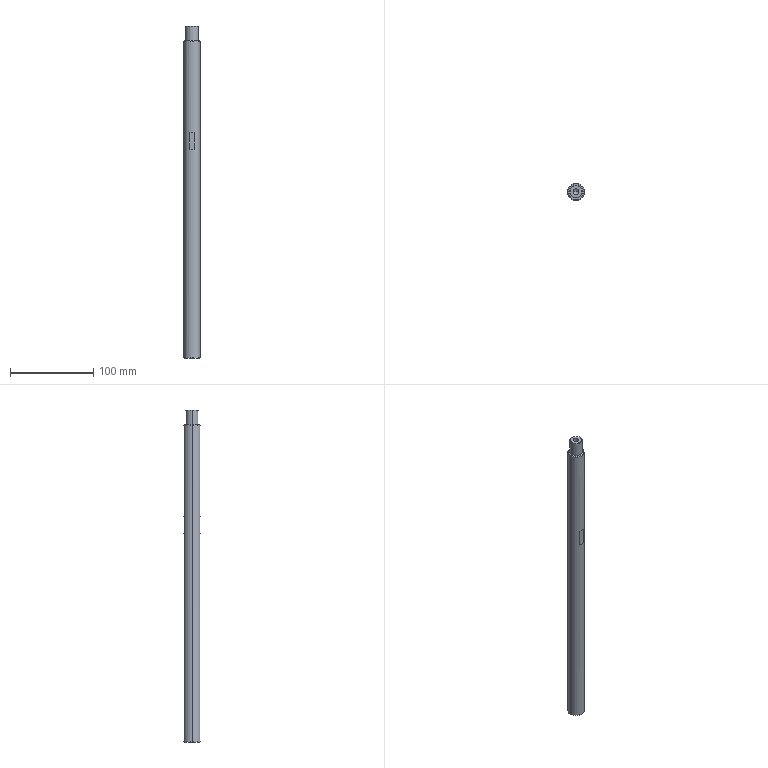Part | STEP file | 11-FG-SJ01611 | 1 solid | 27 faces | box 20 x 20 x 400 mm | volume 121597 mm3 | cone 10 | plane 9 | cylinder 8 | commonest cylinder face diameters 6.8 x4 15 x2 20 x2
STEP:
#1=CARTESIAN_POINT('',(7.,0.,400.));
#2=VERTEX_POINT('',#1);
#3=CARTESIAN_POINT('',(-7.,0.,400.));
#4=VERTEX_POINT('',#3);
#5=CARTESIAN_POINT('',(0.,0.,400.));
#6=DIRECTION('',(0.,0.,1.));
#7=DIRECTION('',(1.,0.,0.));
#8=AXIS2_PLACEMENT_3D('',#5,#6,#7);
#9=CIRCLE('',#8,7.);
#10=EDGE_CURVE('',#2,#4,#9,.T.);
#11=ORIENTED_EDGE('',*,*,#10,.F.);
#12=CARTESIAN_POINT('',(7.5,0.,399.5));
#13=VERTEX_POINT('',#12);
#14=CARTESIAN_POINT('',(7.,0.,400.));
#15=DIRECTION('',(0.7071,0.,-0.7071));
#16=VECTOR('',#15,1000.);
#17=LINE('',#14,#16);
#18=EDGE_CURVE('',#2,#13,#17,.T.);
#19=ORIENTED_EDGE('',*,*,#18,.T.);
#20=CARTESIAN_POINT('',(-7.5,0.,399.5));
#21=VERTEX_POINT('',#20);
#22=CARTESIAN_POINT('',(0.,0.,399.5));
#23=DIRECTION('',(0.,0.,-1.));
#24=DIRECTION('',(1.,0.,0.));
#25=AXIS2_PLACEMENT_3D('',#22,#23,#24);
#26=CIRCLE('',#25,7.5);
#27=EDGE_CURVE('',#21,#13,#26,.T.);
#28=ORIENTED_EDGE('',*,*,#27,.F.);
#29=CARTESIAN_POINT('',(-7.,0.,400.));
#30=DIRECTION('',(-0.7071,0.,-0.7071));
#31=VECTOR('',#30,1000.);
#32=LINE('',#29,#31);
#33=EDGE_CURVE('',#4,#21,#32,.T.);
#34=ORIENTED_EDGE('',*,*,#33,.F.);
#35=EDGE_LOOP('',(#11,#19,#28,#34));
#36=FACE_OUTER_BOUND('',#35,.T.);
#37=CARTESIAN_POINT('',(0.,0.,400.));
#38=DIRECTION('',(0.,0.,-1.));
#39=DIRECTION('',(-1.,0.,0.));
#40=AXIS2_PLACEMENT_3D('',#37,#38,#39);
#41=CONICAL_SURFACE('',#40,7.,0.7854);
#42=ADVANCED_FACE('',(#36),#41,.T.);
#43=CARTESIAN_POINT('',(-9.5,0.,0.));
#44=VERTEX_POINT('',#43);
#45=CARTESIAN_POINT('',(9.5,0.,0.));
#46=VERTEX_POINT('',#45);
#47=CARTESIAN_POINT('',(0.,0.,0.));
#48=DIRECTION('',(0.,0.,-1.));
#49=DIRECTION('',(1.,0.,0.));
#50=AXIS2_PLACEMENT_3D('',#47,#48,#49);
#51=CIRCLE('',#50,9.5);
#52=EDGE_CURVE('',#44,#46,#51,.T.);
#53=ORIENTED_EDGE('',*,*,#52,.F.);
#54=CARTESIAN_POINT('',(-10.,0.,0.5));
#55=VERTEX_POINT('',#54);
#56=CARTESIAN_POINT('',(-10.,0.,0.5));
#57=DIRECTION('',(-0.7071,0.,0.7071));
#58=VECTOR('',#57,1000.);
#59=LINE('',#56,#58);
#60=EDGE_CURVE('',#44,#55,#59,.T.);
#61=ORIENTED_EDGE('',*,*,#60,.T.);
#62=CARTESIAN_POINT('',(10.,0.,0.5));
#63=VERTEX_POINT('',#62);
#64=CARTESIAN_POINT('',(0.,0.,0.5));
#65=DIRECTION('',(0.,0.,1.));
#66=DIRECTION('',(1.,0.,0.));
#67=AXIS2_PLACEMENT_3D('',#64,#65,#66);
#68=CIRCLE('',#67,10.);
#69=EDGE_CURVE('',#63,#55,#68,.T.);
#70=ORIENTED_EDGE('',*,*,#69,.F.);
#71=CARTESIAN_POINT('',(10.,0.,0.5));
#72=DIRECTION('',(0.7071,0.,0.7071));
#73=VECTOR('',#72,1000.);
#74=LINE('',#71,#73);
#75=EDGE_CURVE('',#46,#63,#74,.T.);
#76=ORIENTED_EDGE('',*,*,#75,.F.);
#77=EDGE_LOOP('',(#53,#61,#70,#76));
#78=FACE_OUTER_BOUND('',#77,.T.);
#79=CARTESIAN_POINT('',(0.,0.,0.5));
#80=DIRECTION('',(0.,0.,1.));
#81=DIRECTION('',(1.,0.,0.));
#82=AXIS2_PLACEMENT_3D('',#79,#80,#81);
#83=CONICAL_SURFACE('',#82,10.,0.7854);
#84=ADVANCED_FACE('',(#78),#83,.T.);
#85=CARTESIAN_POINT('',(9.5,0.,382.));
#86=VERTEX_POINT('',#85);
#87=CARTESIAN_POINT('',(-9.5,0.,382.));
#88=VERTEX_POINT('',#87);
#89=CARTESIAN_POINT('',(0.,0.,382.));
#90=DIRECTION('',(0.,0.,1.));
#91=DIRECTION('',(1.,0.,0.));
#92=AXIS2_PLACEMENT_3D('',#89,#90,#91);
#93=CIRCLE('',#92,9.5);
#94=EDGE_CURVE('',#86,#88,#93,.T.);
#95=ORIENTED_EDGE('',*,*,#94,.F.);
#96=CARTESIAN_POINT('',(10.,0.,381.5));
#97=VERTEX_POINT('',#96);
#98=CARTESIAN_POINT('',(9.5,0.,382.));
#99=DIRECTION('',(0.7071,0.,-0.7071));
#100=VECTOR('',#99,1000.);
#101=LINE('',#98,#100);
#102=EDGE_CURVE('',#86,#97,#101,.T.);
#103=ORIENTED_EDGE('',*,*,#102,.T.);
#104=CARTESIAN_POINT('',(-10.,0.,381.5));
#105=VERTEX_POINT('',#104);
#106=CARTESIAN_POINT('',(0.,0.,381.5));
#107=DIRECTION('',(0.,0.,-1.));
#108=DIRECTION('',(1.,0.,0.));
#109=AXIS2_PLACEMENT_3D('',#106,#107,#108);
#110=CIRCLE('',#109,10.);
#111=EDGE_CURVE('',#105,#97,#110,.T.);
#112=ORIENTED_EDGE('',*,*,#111,.F.);
#113=CARTESIAN_POINT('',(-9.5,0.,382.));
#114=DIRECTION('',(-0.7071,0.,-0.7071));
#115=VECTOR('',#114,1000.);
#116=LINE('',#113,#115);
#117=EDGE_CURVE('',#88,#105,#116,.T.);
#118=ORIENTED_EDGE('',*,*,#117,.F.);
#119=EDGE_LOOP('',(#95,#103,#112,#118));
#120=FACE_OUTER_BOUND('',#119,.T.);
#121=CARTESIAN_POINT('',(0.,0.,382.));
#122=DIRECTION('',(0.,0.,-1.));
#123=DIRECTION('',(-1.,0.,0.));
#124=AXIS2_PLACEMENT_3D('',#121,#122,#123);
#125=CONICAL_SURFACE('',#124,9.5,0.7854);
#126=ADVANCED_FACE('',(#120),#125,.T.);
#127=CARTESIAN_POINT('',(-3.4,0.,380.2));
#128=VERTEX_POINT('',#127);
#129=CARTESIAN_POINT('',(3.4,0.,380.2));
#130=VERTEX_POINT('',#129);
#131=CARTESIAN_POINT('',(0.,0.,380.2));
#132=DIRECTION('',(0.,0.,1.));
#133=DIRECTION('',(1.,0.,0.));
#134=AXIS2_PLACEMENT_3D('',#131,#132,#133);
#135=CIRCLE('',#134,3.4);
#136=EDGE_CURVE('',#128,#130,#135,.T.);
#137=ORIENTED_EDGE('',*,*,#136,.F.);
#138=CARTESIAN_POINT('',(-3.4,0.,400.));
#139=VERTEX_POINT('',#138);
#140=CARTESIAN_POINT('',(-3.4,0.,400.));
#141=DIRECTION('',(0.,0.,1.));
#142=VECTOR('',#141,1000.);
#143=LINE('',#140,#142);
#144=EDGE_CURVE('',#128,#139,#143,.T.);
#145=ORIENTED_EDGE('',*,*,#144,.T.);
#146=CARTESIAN_POINT('',(3.4,0.,400.));
#147=VERTEX_POINT('',#146);
#148=CARTESIAN_POINT('',(0.,0.,400.));
#149=DIRECTION('',(0.,0.,1.));
#150=DIRECTION('',(1.,0.,0.));
#151=AXIS2_PLACEMENT_3D('',#148,#149,#150);
#152=CIRCLE('',#151,3.4);
#153=EDGE_CURVE('',#139,#147,#152,.T.);
#154=ORIENTED_EDGE('',*,*,#153,.T.);
#155=CARTESIAN_POINT('',(3.4,0.,400.));
#156=DIRECTION('',(0.,0.,1.));
#157=VECTOR('',#156,1000.);
#158=LINE('',#155,#157);
#159=EDGE_CURVE('',#130,#147,#158,.T.);
#160=ORIENTED_EDGE('',*,*,#159,.F.);
#161=EDGE_LOOP('',(#137,#145,#154,#160));
#162=FACE_OUTER_BOUND('',#161,.T.);
#163=CARTESIAN_POINT('',(0.,0.,400.));
#164=DIRECTION('',(0.,0.,1.));
#165=DIRECTION('',(1.,0.,0.));
#166=AXIS2_PLACEMENT_3D('',#163,#164,#165);
#167=CYLINDRICAL_SURFACE('',#166,3.4);
#168=ADVANCED_FACE('',(#162),#167,.F.);
#169=CARTESIAN_POINT('',(0.,0.,378.157));
#170=VERTEX_POINT('',#169);
#171=CARTESIAN_POINT('',(3.4,0.,380.2));
#172=DIRECTION('',(0.8572,0.,0.515));
#173=VECTOR('',#172,1000.);
#174=LINE('',#171,#173);
#175=EDGE_CURVE('',#170,#130,#174,.T.);
#176=ORIENTED_EDGE('',*,*,#175,.F.);
#177=CARTESIAN_POINT('',(-3.4,0.,380.2));
#178=DIRECTION('',(-0.8572,0.,0.515));
#179=VECTOR('',#178,1000.);
#180=LINE('',#177,#179);
#181=EDGE_CURVE('',#170,#128,#180,.T.);
#182=ORIENTED_EDGE('',*,*,#181,.T.);
#183=ORIENTED_EDGE('',*,*,#136,.T.);
#184=EDGE_LOOP('',(#176,#182,#183));
#185=FACE_OUTER_BOUND('',#184,.T.);
#186=CARTESIAN_POINT('',(0.,0.,380.2));
#187=DIRECTION('',(0.,0.,1.));
#188=DIRECTION('',(1.,0.,0.));
#189=AXIS2_PLACEMENT_3D('',#186,#187,#188);
#190=CONICAL_SURFACE('',#189,3.4,1.03);
#191=ADVANCED_FACE('',(#185),#190,.F.);
#192=CARTESIAN_POINT('',(7.5,0.,382.));
#193=VERTEX_POINT('',#192);
#194=CARTESIAN_POINT('',(-7.5,0.,382.));
#195=VERTEX_POINT('',#194);
#196=CARTESIAN_POINT('',(0.,0.,382.));
#197=DIRECTION('',(0.,0.,1.));
#198=DIRECTION('',(1.,0.,0.));
#199=AXIS2_PLACEMENT_3D('',#196,#197,#198);
#200=CIRCLE('',#199,7.5);
#201=EDGE_CURVE('',#193,#195,#200,.T.);
#202=ORIENTED_EDGE('',*,*,#201,.T.);
#203=CARTESIAN_POINT('',(-7.5,0.,382.));
#204=DIRECTION('',(0.,0.,1.));
#205=VECTOR('',#204,1000.);
#206=LINE('',#203,#205);
#207=EDGE_CURVE('',#195,#21,#206,.T.);
#208=ORIENTED_EDGE('',*,*,#207,.T.);
#209=ORIENTED_EDGE('',*,*,#27,.T.);
#210=CARTESIAN_POINT('',(7.5,0.,382.));
#211=DIRECTION('',(0.,0.,1.));
#212=VECTOR('',#211,1000.);
#213=LINE('',#210,#212);
#214=EDGE_CURVE('',#193,#13,#213,.T.);
#215=ORIENTED_EDGE('',*,*,#214,.F.);
#216=EDGE_LOOP('',(#202,#208,#209,#215));
#217=FACE_OUTER_BOUND('',#216,.T.);
#218=CARTESIAN_POINT('',(0.,0.,382.));
#219=DIRECTION('',(0.,0.,1.));
#220=DIRECTION('',(1.,0.,0.));
#221=AXIS2_PLACEMENT_3D('',#218,#219,#220);
#222=CYLINDRICAL_SURFACE('',#221,7.5);
#223=ADVANCED_FACE('',(#217),#222,.T.);
#224=CARTESIAN_POINT('',(3.4,0.,19.8));
#225=VERTEX_POINT('',#224);
#226=CARTESIAN_POINT('',(-3.4,0.,19.8));
#227=VERTEX_POINT('',#226);
#228=CARTESIAN_POINT('',(0.,0.,19.8));
#229=DIRECTION('',(0.,0.,-1.));
#230=DIRECTION('',(-1.,0.,0.));
#231=AXIS2_PLACEMENT_3D('',#228,#229,#230);
#232=CIRCLE('',#231,3.4);
#233=EDGE_CURVE('',#225,#227,#232,.T.);
#234=ORIENTED_EDGE('',*,*,#233,.F.);
#235=CARTESIAN_POINT('',(3.4,0.,0.));
#236=VERTEX_POINT('',#235);
#237=CARTESIAN_POINT('',(3.4,0.,0.));
#238=DIRECTION('',(0.,0.,-1.));
#239=VECTOR('',#238,1000.);
#240=LINE('',#237,#239);
#241=EDGE_CURVE('',#225,#236,#240,.T.);
#242=ORIENTED_EDGE('',*,*,#241,.T.);
#243=CARTESIAN_POINT('',(-3.4,0.,0.));
#244=VERTEX_POINT('',#243);
#245=CARTESIAN_POINT('',(0.,0.,0.));
#246=DIRECTION('',(0.,0.,-1.));
#247=DIRECTION('',(-1.,0.,0.));
#248=AXIS2_PLACEMENT_3D('',#245,#246,#247);
#249=CIRCLE('',#248,3.4);
#250=EDGE_CURVE('',#236,#244,#249,.T.);
#251=ORIENTED_EDGE('',*,*,#250,.T.);
#252=CARTESIAN_POINT('',(-3.4,0.,0.));
#253=DIRECTION('',(0.,0.,-1.));
#254=VECTOR('',#253,1000.);
#255=LINE('',#252,#254);
#256=EDGE_CURVE('',#227,#244,#255,.T.);
#257=ORIENTED_EDGE('',*,*,#256,.F.);
#258=EDGE_LOOP('',(#234,#242,#251,#257));
#259=FACE_OUTER_BOUND('',#258,.T.);
#260=CARTESIAN_POINT('',(0.,0.,0.));
#261=DIRECTION('',(0.,0.,-1.));
#262=DIRECTION('',(-1.,0.,0.));
#263=AXIS2_PLACEMENT_3D('',#260,#261,#262);
#264=CYLINDRICAL_SURFACE('',#263,3.4);
#265=ADVANCED_FACE('',(#259),#264,.F.);
#266=CARTESIAN_POINT('',(0.,0.,21.843));
#267=VERTEX_POINT('',#266);
#268=CARTESIAN_POINT('',(-3.4,0.,19.8));
#269=DIRECTION('',(-0.8572,0.,-0.515));
#270=VECTOR('',#269,1000.);
#271=LINE('',#268,#270);
#272=EDGE_CURVE('',#267,#227,#271,.T.);
#273=ORIENTED_EDGE('',*,*,#272,.F.);
#274=CARTESIAN_POINT('',(3.4,0.,19.8));
#275=DIRECTION('',(0.8572,0.,-0.515));
#276=VECTOR('',#275,1000.);
#277=LINE('',#274,#276);
#278=EDGE_CURVE('',#267,#225,#277,.T.);
#279=ORIENTED_EDGE('',*,*,#278,.T.);
#280=ORIENTED_EDGE('',*,*,#233,.T.);
#281=EDGE_LOOP('',(#273,#279,#280));
#282=FACE_OUTER_BOUND('',#281,.T.);
#283=CARTESIAN_POINT('',(0.,0.,19.8));
#284=DIRECTION('',(0.,0.,-1.));
#285=DIRECTION('',(-1.,0.,0.));
#286=AXIS2_PLACEMENT_3D('',#283,#284,#285);
#287=CONICAL_SURFACE('',#286,3.4,1.03);
#288=ADVANCED_FACE('',(#282),#287,.F.);
#289=CARTESIAN_POINT('',(3.122,9.5,251.5));
#290=VERTEX_POINT('',#289);
#291=CARTESIAN_POINT('',(-3.122,9.5,251.5));
#292=VERTEX_POINT('',#291);
#293=CARTESIAN_POINT('',(0.,0.,251.5));
#294=DIRECTION('',(0.,0.,1.));
#295=DIRECTION('',(1.,0.,0.));
#296=AXIS2_PLACEMENT_3D('',#293,#294,#295);
#297=CIRCLE('',#296,10.);
#298=EDGE_CURVE('',#290,#292,#297,.T.);
#299=ORIENTED_EDGE('',*,*,#298,.F.);
#300=CARTESIAN_POINT('',(3.122,9.5,271.5));
#301=VERTEX_POINT('',#300);
#302=CARTESIAN_POINT('',(3.122,9.5,251.5));
#303=DIRECTION('',(0.,0.,1.));
#304=VECTOR('',#303,1000.);
#305=LINE('',#302,#304);
#306=EDGE_CURVE('',#290,#301,#305,.T.);
#307=ORIENTED_EDGE('',*,*,#306,.T.);
#308=CARTESIAN_POINT('',(-3.122,9.5,271.5));
#309=VERTEX_POINT('',#308);
#310=CARTESIAN_POINT('',(0.,0.,271.5));
#311=DIRECTION('',(0.,0.,1.));
#312=DIRECTION('',(1.,0.,0.));
#313=AXIS2_PLACEMENT_3D('',#310,#311,#312);
#314=CIRCLE('',#313,10.);
#315=EDGE_CURVE('',#301,#309,#314,.T.);
#316=ORIENTED_EDGE('',*,*,#315,.T.);
#317=CARTESIAN_POINT('',(-3.122,9.5,251.5));
#318=DIRECTION('',(0.,0.,1.));
#319=VECTOR('',#318,1000.);
#320=LINE('',#317,#319);
#321=EDGE_CURVE('',#292,#309,#320,.T.);
#322=ORIENTED_EDGE('',*,*,#321,.F.);
#323=EDGE_LOOP('',(#299,#307,#316,#322));
#324=FACE_BOUND('',#323,.T.);
#325=ORIENTED_EDGE('',*,*,#111,.T.);
#326=CARTESIAN_POINT('',(10.,0.,400.));
#327=DIRECTION('',(0.,0.,-1.));
#328=VECTOR('',#327,1000.);
#329=LINE('',#326,#328);
#330=EDGE_CURVE('',#97,#63,#329,.T.);
#331=ORIENTED_EDGE('',*,*,#330,.T.);
#332=ORIENTED_EDGE('',*,*,#69,.T.);
#333=CARTESIAN_POINT('',(-10.,0.,400.));
#334=DIRECTION('',(0.,0.,-1.));
#335=VECTOR('',#334,1000.);
#336=LINE('',#333,#335);
#337=EDGE_CURVE('',#105,#55,#336,.T.);
#338=ORIENTED_EDGE('',*,*,#337,.F.);
#339=EDGE_LOOP('',(#325,#331,#332,#338));
#340=FACE_OUTER_BOUND('',#339,.T.);
#341=CARTESIAN_POINT('',(0.,0.,400.));
#342=DIRECTION('',(0.,0.,-1.));
#343=DIRECTION('',(-1.,0.,0.));
#344=AXIS2_PLACEMENT_3D('',#341,#342,#343);
#345=CYLINDRICAL_SURFACE('',#344,10.);
#346=ADVANCED_FACE('',(#324,#340),#345,.T.);
#347=ORIENTED_EDGE('',*,*,#330,.F.);
#348=CARTESIAN_POINT('',(0.,0.,381.5));
#349=DIRECTION('',(0.,0.,-1.));
#350=DIRECTION('',(1.,0.,0.));
#351=AXIS2_PLACEMENT_3D('',#348,#349,#350);
#352=CIRCLE('',#351,10.);
#353=EDGE_CURVE('',#97,#105,#352,.T.);
#354=ORIENTED_EDGE('',*,*,#353,.T.);
#355=ORIENTED_EDGE('',*,*,#337,.T.);
#356=CARTESIAN_POINT('',(0.,0.,0.5));
#357=DIRECTION('',(0.,0.,1.));
#358=DIRECTION('',(1.,0.,0.));
#359=AXIS2_PLACEMENT_3D('',#356,#357,#358);
#360=CIRCLE('',#359,10.);
#361=EDGE_CURVE('',#55,#63,#360,.T.);
#362=ORIENTED_EDGE('',*,*,#361,.T.);
#363=EDGE_LOOP('',(#347,#354,#355,#362));
#364=FACE_OUTER_BOUND('',#363,.T.);
#365=CARTESIAN_POINT('',(-3.122,-9.5,251.5));
#366=VERTEX_POINT('',#365);
#367=CARTESIAN_POINT('',(3.122,-9.5,251.5));
#368=VERTEX_POINT('',#367);
#369=CARTESIAN_POINT('',(0.,0.,251.5));
#370=DIRECTION('',(0.,0.,1.));
#371=DIRECTION('',(1.,0.,0.));
#372=AXIS2_PLACEMENT_3D('',#369,#370,#371);
#373=CIRCLE('',#372,10.);
#374=EDGE_CURVE('',#366,#368,#373,.T.);
#375=ORIENTED_EDGE('',*,*,#374,.F.);
#376=CARTESIAN_POINT('',(-3.122,-9.5,271.5));
#377=VERTEX_POINT('',#376);
#378=CARTESIAN_POINT('',(-3.122,-9.5,251.5));
#379=DIRECTION('',(0.,0.,1.));
#380=VECTOR('',#379,1000.);
#381=LINE('',#378,#380);
#382=EDGE_CURVE('',#366,#377,#381,.T.);
#383=ORIENTED_EDGE('',*,*,#382,.T.);
#384=CARTESIAN_POINT('',(3.122,-9.5,271.5));
#385=VERTEX_POINT('',#384);
#386=CARTESIAN_POINT('',(0.,0.,271.5));
#387=DIRECTION('',(0.,0.,1.));
#388=DIRECTION('',(1.,0.,0.));
#389=AXIS2_PLACEMENT_3D('',#386,#387,#388);
#390=CIRCLE('',#389,10.);
#391=EDGE_CURVE('',#377,#385,#390,.T.);
#392=ORIENTED_EDGE('',*,*,#391,.T.);
#393=CARTESIAN_POINT('',(3.122,-9.5,251.5));
#394=DIRECTION('',(0.,0.,1.));
#395=VECTOR('',#394,1000.);
#396=LINE('',#393,#395);
#397=EDGE_CURVE('',#368,#385,#396,.T.);
#398=ORIENTED_EDGE('',*,*,#397,.F.);
#399=EDGE_LOOP('',(#375,#383,#392,#398));
#400=FACE_BOUND('',#399,.T.);
#401=CARTESIAN_POINT('',(0.,0.,400.));
#402=DIRECTION('',(0.,0.,-1.));
#403=DIRECTION('',(-1.,0.,0.));
#404=AXIS2_PLACEMENT_3D('',#401,#402,#403);
#405=CYLINDRICAL_SURFACE('',#404,10.);
#406=ADVANCED_FACE('',(#364,#400),#405,.T.);
#407=CARTESIAN_POINT('',(0.,0.,0.));
#408=DIRECTION('',(0.,0.,-1.));
#409=DIRECTION('',(1.,0.,0.));
#410=AXIS2_PLACEMENT_3D('',#407,#408,#409);
#411=CIRCLE('',#410,9.5);
#412=EDGE_CURVE('',#46,#44,#411,.T.);
#413=ORIENTED_EDGE('',*,*,#412,.T.);
#414=ORIENTED_EDGE('',*,*,#52,.T.);
#415=EDGE_LOOP('',(#413,#414));
#416=FACE_OUTER_BOUND('',#415,.T.);
#417=CARTESIAN_POINT('',(0.,0.,0.));
#418=DIRECTION('',(0.,0.,-1.));
#419=DIRECTION('',(-1.,0.,0.));
#420=AXIS2_PLACEMENT_3D('',#417,#418,#419);
#421=CIRCLE('',#420,3.4);
#422=EDGE_CURVE('',#244,#236,#421,.T.);
#423=ORIENTED_EDGE('',*,*,#422,.F.);
#424=ORIENTED_EDGE('',*,*,#250,.F.);
#425=EDGE_LOOP('',(#423,#424));
#426=FACE_BOUND('',#425,.T.);
#427=CARTESIAN_POINT('',(0.,0.,0.));
#428=DIRECTION('',(0.,0.,1.));
#429=DIRECTION('',(1.,0.,0.));
#430=AXIS2_PLACEMENT_3D('',#427,#428,#429);
#431=PLANE('',#430);
#432=ADVANCED_FACE('',(#416,#426),#431,.F.);
#433=CARTESIAN_POINT('',(-3.122,9.5,271.5));
#434=DIRECTION('',(1.,0.,0.));
#435=VECTOR('',#434,1000.);
#436=LINE('',#433,#435);
#437=EDGE_CURVE('',#309,#301,#436,.T.);
#438=ORIENTED_EDGE('',*,*,#437,.T.);
#439=ORIENTED_EDGE('',*,*,#306,.F.);
#440=CARTESIAN_POINT('',(-3.122,9.5,251.5));
#441=DIRECTION('',(1.,0.,0.));
#442=VECTOR('',#441,1000.);
#443=LINE('',#440,#442);
#444=EDGE_CURVE('',#292,#290,#443,.T.);
#445=ORIENTED_EDGE('',*,*,#444,.F.);
#446=ORIENTED_EDGE('',*,*,#321,.T.);
#447=EDGE_LOOP('',(#438,#439,#445,#446));
#448=FACE_OUTER_BOUND('',#447,.T.);
#449=CARTESIAN_POINT('',(-3.122,9.5,251.5));
#450=DIRECTION('',(0.,-1.,0.));
#451=DIRECTION('',(0.,0.,-1.));
#452=AXIS2_PLACEMENT_3D('',#449,#450,#451);
#453=PLANE('',#452);
#454=ADVANCED_FACE('',(#448),#453,.F.);
#455=ORIENTED_EDGE('',*,*,#298,.T.);
#456=ORIENTED_EDGE('',*,*,#444,.T.);
#457=EDGE_LOOP('',(#455,#456));
#458=FACE_OUTER_BOUND('',#457,.T.);
#459=CARTESIAN_POINT('',(0.,0.,251.5));
#460=DIRECTION('',(0.,0.,1.));
#461=DIRECTION('',(1.,0.,0.));
#462=AXIS2_PLACEMENT_3D('',#459,#460,#461);
#463=PLANE('',#462);
#464=ADVANCED_FACE('',(#458),#463,.T.);
#465=ORIENTED_EDGE('',*,*,#315,.F.);
#466=ORIENTED_EDGE('',*,*,#437,.F.);
#467=EDGE_LOOP('',(#465,#466));
#468=FACE_OUTER_BOUND('',#467,.T.);
#469=CARTESIAN_POINT('',(0.,0.,271.5));
#470=DIRECTION('',(0.,0.,1.));
#471=DIRECTION('',(1.,0.,0.));
#472=AXIS2_PLACEMENT_3D('',#469,#470,#471);
#473=PLANE('',#472);
#474=ADVANCED_FACE('',(#468),#473,.F.);
#475=CARTESIAN_POINT('',(-3.122,-9.5,271.5));
#476=DIRECTION('',(-1.,0.,0.));
#477=VECTOR('',#476,1000.);
#478=LINE('',#475,#477);
#479=EDGE_CURVE('',#385,#377,#478,.T.);
#480=ORIENTED_EDGE('',*,*,#479,.T.);
#481=ORIENTED_EDGE('',*,*,#382,.F.);
#482=CARTESIAN_POINT('',(-3.122,-9.5,251.5));
#483=DIRECTION('',(-1.,0.,0.));
#484=VECTOR('',#483,1000.);
#485=LINE('',#482,#484);
#486=EDGE_CURVE('',#368,#366,#485,.T.);
#487=ORIENTED_EDGE('',*,*,#486,.F.);
#488=ORIENTED_EDGE('',*,*,#397,.T.);
#489=EDGE_LOOP('',(#480,#481,#487,#488));
#490=FACE_OUTER_BOUND('',#489,.T.);
#491=CARTESIAN_POINT('',(-3.122,-9.5,251.5));
#492=DIRECTION('',(0.,1.,0.));
#493=DIRECTION('',(0.,0.,1.));
#494=AXIS2_PLACEMENT_3D('',#491,#492,#493);
#495=PLANE('',#494);
#496=ADVANCED_FACE('',(#490),#495,.F.);
#497=ORIENTED_EDGE('',*,*,#374,.T.);
#498=ORIENTED_EDGE('',*,*,#486,.T.);
#499=EDGE_LOOP('',(#497,#498));
#500=FACE_OUTER_BOUND('',#499,.T.);
#501=CARTESIAN_POINT('',(0.,0.,251.5));
#502=DIRECTION('',(0.,0.,1.));
#503=DIRECTION('',(1.,0.,0.));
#504=AXIS2_PLACEMENT_3D('',#501,#502,#503);
#505=PLANE('',#504);
#506=ADVANCED_FACE('',(#500),#505,.T.);
#507=ORIENTED_EDGE('',*,*,#391,.F.);
#508=ORIENTED_EDGE('',*,*,#479,.F.);
#509=EDGE_LOOP('',(#507,#508));
#510=FACE_OUTER_BOUND('',#509,.T.);
#511=CARTESIAN_POINT('',(0.,0.,271.5));
#512=DIRECTION('',(0.,0.,1.));
#513=DIRECTION('',(1.,0.,0.));
#514=AXIS2_PLACEMENT_3D('',#511,#512,#513);
#515=PLANE('',#514);
#516=ADVANCED_FACE('',(#510),#515,.F.);
#517=ORIENTED_EDGE('',*,*,#278,.F.);
#518=ORIENTED_EDGE('',*,*,#272,.T.);
#519=CARTESIAN_POINT('',(0.,0.,19.8));
#520=DIRECTION('',(0.,0.,-1.));
#521=DIRECTION('',(-1.,0.,0.));
#522=AXIS2_PLACEMENT_3D('',#519,#520,#521);
#523=CIRCLE('',#522,3.4);
#524=EDGE_CURVE('',#227,#225,#523,.T.);
#525=ORIENTED_EDGE('',*,*,#524,.T.);
#526=EDGE_LOOP('',(#517,#518,#525));
#527=FACE_OUTER_BOUND('',#526,.T.);
#528=CARTESIAN_POINT('',(0.,0.,19.8));
#529=DIRECTION('',(0.,0.,-1.));
#530=DIRECTION('',(-1.,0.,0.));
#531=AXIS2_PLACEMENT_3D('',#528,#529,#530);
#532=CONICAL_SURFACE('',#531,3.4,1.03);
#533=ADVANCED_FACE('',(#527),#532,.F.);
#534=ORIENTED_EDGE('',*,*,#241,.F.);
#535=ORIENTED_EDGE('',*,*,#524,.F.);
#536=ORIENTED_EDGE('',*,*,#256,.T.);
#537=ORIENTED_EDGE('',*,*,#422,.T.);
#538=EDGE_LOOP('',(#534,#535,#536,#537));
#539=FACE_OUTER_BOUND('',#538,.T.);
#540=CARTESIAN_POINT('',(0.,0.,0.));
#541=DIRECTION('',(0.,0.,-1.));
#542=DIRECTION('',(-1.,0.,0.));
#543=AXIS2_PLACEMENT_3D('',#540,#541,#542);
#544=CYLINDRICAL_SURFACE('',#543,3.4);
#545=ADVANCED_FACE('',(#539),#544,.F.);
#546=CARTESIAN_POINT('',(0.,0.,382.));
#547=DIRECTION('',(0.,0.,1.));
#548=DIRECTION('',(1.,0.,0.));
#549=AXIS2_PLACEMENT_3D('',#546,#547,#548);
#550=CIRCLE('',#549,9.5);
#551=EDGE_CURVE('',#88,#86,#550,.T.);
#552=ORIENTED_EDGE('',*,*,#551,.T.);
#553=ORIENTED_EDGE('',*,*,#94,.T.);
#554=EDGE_LOOP('',(#552,#553));
#555=FACE_OUTER_BOUND('',#554,.T.);
#556=ORIENTED_EDGE('',*,*,#201,.F.);
#557=CARTESIAN_POINT('',(0.,0.,382.));
#558=DIRECTION('',(0.,0.,1.));
#559=DIRECTION('',(1.,0.,0.));
#560=AXIS2_PLACEMENT_3D('',#557,#558,#559);
#561=CIRCLE('',#560,7.5);
#562=EDGE_CURVE('',#195,#193,#561,.T.);
#563=ORIENTED_EDGE('',*,*,#562,.F.);
#564=EDGE_LOOP('',(#556,#563));
#565=FACE_BOUND('',#564,.T.);
#566=CARTESIAN_POINT('',(0.,0.,382.));
#567=DIRECTION('',(0.,0.,1.));
#568=DIRECTION('',(1.,0.,0.));
#569=AXIS2_PLACEMENT_3D('',#566,#567,#568);
#570=PLANE('',#569);
#571=ADVANCED_FACE('',(#555,#565),#570,.T.);
#572=ORIENTED_EDGE('',*,*,#207,.F.);
#573=ORIENTED_EDGE('',*,*,#562,.T.);
#574=ORIENTED_EDGE('',*,*,#214,.T.);
#575=CARTESIAN_POINT('',(0.,0.,399.5));
#576=DIRECTION('',(0.,0.,-1.));
#577=DIRECTION('',(1.,0.,0.));
#578=AXIS2_PLACEMENT_3D('',#575,#576,#577);
#579=CIRCLE('',#578,7.5);
#580=EDGE_CURVE('',#13,#21,#579,.T.);
#581=ORIENTED_EDGE('',*,*,#580,.T.);
#582=EDGE_LOOP('',(#572,#573,#574,#581));
#583=FACE_OUTER_BOUND('',#582,.T.);
#584=CARTESIAN_POINT('',(0.,0.,382.));
#585=DIRECTION('',(0.,0.,1.));
#586=DIRECTION('',(1.,0.,0.));
#587=AXIS2_PLACEMENT_3D('',#584,#585,#586);
#588=CYLINDRICAL_SURFACE('',#587,7.5);
#589=ADVANCED_FACE('',(#583),#588,.T.);
#590=ORIENTED_EDGE('',*,*,#181,.F.);
#591=ORIENTED_EDGE('',*,*,#175,.T.);
#592=CARTESIAN_POINT('',(0.,0.,380.2));
#593=DIRECTION('',(0.,0.,1.));
#594=DIRECTION('',(1.,0.,0.));
#595=AXIS2_PLACEMENT_3D('',#592,#593,#594);
#596=CIRCLE('',#595,3.4);
#597=EDGE_CURVE('',#130,#128,#596,.T.);
#598=ORIENTED_EDGE('',*,*,#597,.T.);
#599=EDGE_LOOP('',(#590,#591,#598));
#600=FACE_OUTER_BOUND('',#599,.T.);
#601=CARTESIAN_POINT('',(0.,0.,380.2));
#602=DIRECTION('',(0.,0.,1.));
#603=DIRECTION('',(1.,0.,0.));
#604=AXIS2_PLACEMENT_3D('',#601,#602,#603);
#605=CONICAL_SURFACE('',#604,3.4,1.03);
#606=ADVANCED_FACE('',(#600),#605,.F.);
#607=ORIENTED_EDGE('',*,*,#144,.F.);
#608=ORIENTED_EDGE('',*,*,#597,.F.);
#609=ORIENTED_EDGE('',*,*,#159,.T.);
#610=CARTESIAN_POINT('',(0.,0.,400.));
#611=DIRECTION('',(0.,0.,1.));
#612=DIRECTION('',(1.,0.,0.));
#613=AXIS2_PLACEMENT_3D('',#610,#611,#612);
#614=CIRCLE('',#613,3.4);
#615=EDGE_CURVE('',#147,#139,#614,.T.);
#616=ORIENTED_EDGE('',*,*,#615,.T.);
#617=EDGE_LOOP('',(#607,#608,#609,#616));
#618=FACE_OUTER_BOUND('',#617,.T.);
#619=CARTESIAN_POINT('',(0.,0.,400.));
#620=DIRECTION('',(0.,0.,1.));
#621=DIRECTION('',(1.,0.,0.));
#622=AXIS2_PLACEMENT_3D('',#619,#620,#621);
#623=CYLINDRICAL_SURFACE('',#622,3.4);
#624=ADVANCED_FACE('',(#618),#623,.F.);
#625=CARTESIAN_POINT('',(0.,0.,400.));
#626=DIRECTION('',(0.,0.,1.));
#627=DIRECTION('',(1.,0.,0.));
#628=AXIS2_PLACEMENT_3D('',#625,#626,#627);
#629=CIRCLE('',#628,7.);
#630=EDGE_CURVE('',#4,#2,#629,.T.);
#631=ORIENTED_EDGE('',*,*,#630,.T.);
#632=ORIENTED_EDGE('',*,*,#10,.T.);
#633=EDGE_LOOP('',(#631,#632));
#634=FACE_OUTER_BOUND('',#633,.T.);
#635=ORIENTED_EDGE('',*,*,#615,.F.);
#636=ORIENTED_EDGE('',*,*,#153,.F.);
#637=EDGE_LOOP('',(#635,#636));
#638=FACE_BOUND('',#637,.T.);
#639=CARTESIAN_POINT('',(0.,0.,400.));
#640=DIRECTION('',(0.,0.,1.));
#641=DIRECTION('',(1.,0.,0.));
#642=AXIS2_PLACEMENT_3D('',#639,#640,#641);
#643=PLANE('',#642);
#644=ADVANCED_FACE('',(#634,#638),#643,.T.);
#645=ORIENTED_EDGE('',*,*,#102,.F.);
#646=ORIENTED_EDGE('',*,*,#551,.F.);
#647=ORIENTED_EDGE('',*,*,#117,.T.);
#648=ORIENTED_EDGE('',*,*,#353,.F.);
#649=EDGE_LOOP('',(#645,#646,#647,#648));
#650=FACE_OUTER_BOUND('',#649,.T.);
#651=CARTESIAN_POINT('',(0.,0.,382.));
#652=DIRECTION('',(0.,0.,-1.));
#653=DIRECTION('',(-1.,0.,0.));
#654=AXIS2_PLACEMENT_3D('',#651,#652,#653);
#655=CONICAL_SURFACE('',#654,9.5,0.7854);
#656=ADVANCED_FACE('',(#650),#655,.T.);
#657=ORIENTED_EDGE('',*,*,#60,.F.);
#658=ORIENTED_EDGE('',*,*,#412,.F.);
#659=ORIENTED_EDGE('',*,*,#75,.T.);
#660=ORIENTED_EDGE('',*,*,#361,.F.);
#661=EDGE_LOOP('',(#657,#658,#659,#660));
#662=FACE_OUTER_BOUND('',#661,.T.);
#663=CARTESIAN_POINT('',(0.,0.,0.5));
#664=DIRECTION('',(0.,0.,1.));
#665=DIRECTION('',(1.,0.,0.));
#666=AXIS2_PLACEMENT_3D('',#663,#664,#665);
#667=CONICAL_SURFACE('',#666,10.,0.7854);
#668=ADVANCED_FACE('',(#662),#667,.T.);
#669=ORIENTED_EDGE('',*,*,#18,.F.);
#670=ORIENTED_EDGE('',*,*,#630,.F.);
#671=ORIENTED_EDGE('',*,*,#33,.T.);
#672=ORIENTED_EDGE('',*,*,#580,.F.);
#673=EDGE_LOOP('',(#669,#670,#671,#672));
#674=FACE_OUTER_BOUND('',#673,.T.);
#675=CARTESIAN_POINT('',(0.,0.,400.));
#676=DIRECTION('',(0.,0.,-1.));
#677=DIRECTION('',(-1.,0.,0.));
#678=AXIS2_PLACEMENT_3D('',#675,#676,#677);
#679=CONICAL_SURFACE('',#678,7.,0.7854);
#680=ADVANCED_FACE('',(#674),#679,.T.);
#681=CLOSED_SHELL('',(#42,#84,#126,#168,#191,#223,#265,#288,#346,#406,#432,#454,#464,#474,#496,#506,#516,#533,#545,#571,#589,#606,#624,#644,#656,#668,#680));
#682=MANIFOLD_SOLID_BREP('',#681);
#683=CARTESIAN_POINT('',(0.,0.,0.));
#684=DIRECTION('',(0.,0.,1.));
#685=DIRECTION('',(1.,0.,0.));
#686=AXIS2_PLACEMENT_3D('',#683,#684,#685);
#687=(LENGTH_UNIT()NAMED_UNIT(*)SI_UNIT(.MILLI.,.METRE.));
#688=UNCERTAINTY_MEASURE_WITH_UNIT(LENGTH_MEASURE(0.00001),#687,'','');
#689=(NAMED_UNIT(*)PLANE_ANGLE_UNIT()SI_UNIT($,.RADIAN.));
#690=(NAMED_UNIT(*)SI_UNIT($,.STERADIAN.)SOLID_ANGLE_UNIT());
#691=(GEOMETRIC_REPRESENTATION_CONTEXT(3)GLOBAL_UNCERTAINTY_ASSIGNED_CONTEXT((#688))GLOBAL_UNIT_ASSIGNED_CONTEXT((#687,#689,#690))REPRESENTATION_CONTEXT('',''));
#692=ADVANCED_BREP_SHAPE_REPRESENTATION('',(#682,#686),#691);